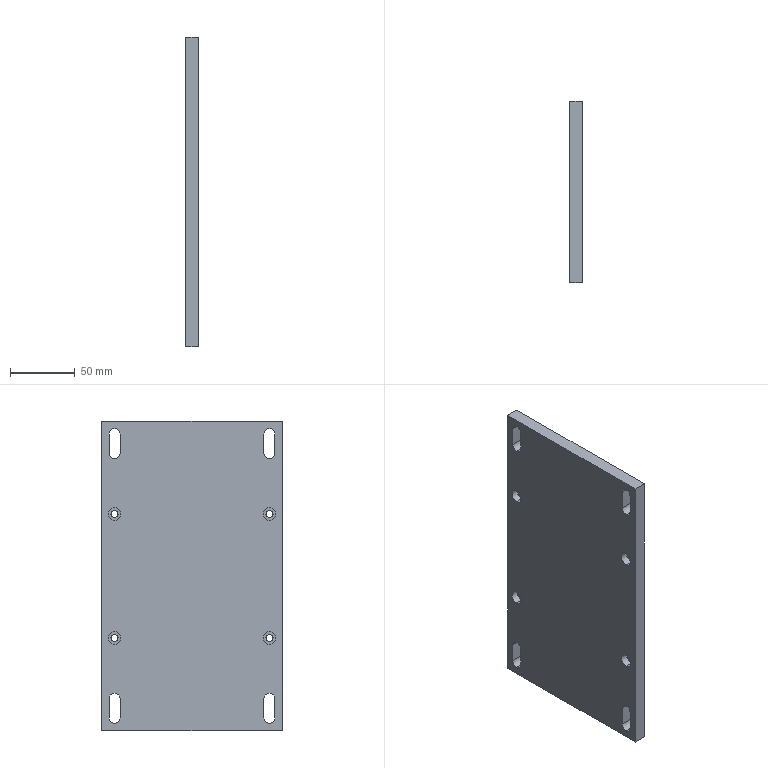Part | STEP file | 06-36 Front-rear dovetail base plate | 1 solid | 46 faces | box 10 x 140 x 240 mm | volume 326475 mm3 | cylinder 28 | plane 18 | commonest cylinder face diameters 8.5 x12 5.5 x8 10 x8